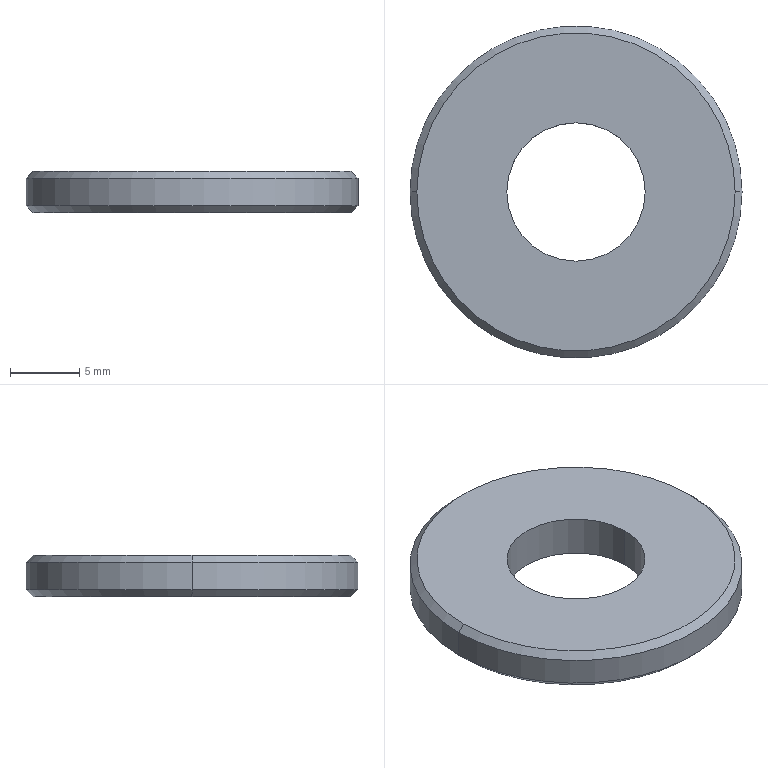Part | STEP file | VALVE_4PARTV11 | 1 solid | 10 faces | box 24 x 24 x 3 mm | volume 1103 mm3 | cone 4 | cylinder 4 | plane 2 | commonest cylinder face diameters 10 x2 24 x2
STEP:
#1=CARTESIAN_POINT('',(0.,0.,0.));
#2=DIRECTION('',(0.,0.,1.));
#3=DIRECTION('',(1.,0.,0.));
#4=AXIS2_PLACEMENT_3D('',#1,#2,#3);
#5=CARTESIAN_POINT('',(11.5,0.,3.));
#6=VERTEX_POINT('',#5);
#7=CARTESIAN_POINT('',(-11.5,0.,3.));
#8=VERTEX_POINT('',#7);
#9=CARTESIAN_POINT('',(0.,0.,3.));
#10=DIRECTION('',(0.,0.,1.));
#11=DIRECTION('',(1.,0.,0.));
#12=AXIS2_PLACEMENT_3D('',#9,#10,#11);
#13=CIRCLE('',#12,11.5);
#14=CARTESIAN_POINT('',(0.,0.,3.));
#15=DIRECTION('',(0.,0.,-1.));
#16=DIRECTION('',(-1.,0.,0.));
#17=AXIS2_PLACEMENT_3D('',#14,#15,#16);
#18=CONICAL_SURFACE('',#17,11.5,0.7854);
#19=CARTESIAN_POINT('',(3.142,0.));
#20=DIRECTION('',(-1.,0.));
#21=VECTOR('',#20,1.);
#22=LINE('',#19,#21);
#23=(GEOMETRIC_REPRESENTATION_CONTEXT(2)PARAMETRIC_REPRESENTATION_CONTEXT()REPRESENTATION_CONTEXT('',''));
#24=DEFINITIONAL_REPRESENTATION('',(#22),#23);
#25=PCURVE('',#18,#24);
#26=CARTESIAN_POINT('',(0.,0.,3.));
#27=DIRECTION('',(0.,0.,1.));
#28=DIRECTION('',(1.,0.,0.));
#29=AXIS2_PLACEMENT_3D('',#26,#27,#28);
#30=PLANE('',#29);
#31=CARTESIAN_POINT('',(0.,0.));
#32=DIRECTION('',(1.,0.));
#33=AXIS2_PLACEMENT_2D('',#31,#32);
#34=CIRCLE('',#33,11.5);
#35=(GEOMETRIC_REPRESENTATION_CONTEXT(2)PARAMETRIC_REPRESENTATION_CONTEXT()REPRESENTATION_CONTEXT('',''));
#36=DEFINITIONAL_REPRESENTATION('',(#34),#35);
#37=PCURVE('',#30,#36);
#38=SURFACE_CURVE('',#13,(#25,#37),.PCURVE_S1.);
#39=EDGE_CURVE('',#6,#8,#38,.T.);
#40=ORIENTED_EDGE('',*,*,#39,.F.);
#41=CARTESIAN_POINT('',(12.,0.,2.5));
#42=VERTEX_POINT('',#41);
#43=CARTESIAN_POINT('',(11.5,0.,3.));
#44=DIRECTION('',(0.7071,0.,-0.7071));
#45=VECTOR('',#44,1.);
#46=LINE('',#43,#45);
#47=CARTESIAN_POINT('',(3.142,0.));
#48=DIRECTION('',(0.,1.));
#49=VECTOR('',#48,1.);
#50=LINE('',#47,#49);
#51=(GEOMETRIC_REPRESENTATION_CONTEXT(2)PARAMETRIC_REPRESENTATION_CONTEXT()REPRESENTATION_CONTEXT('',''));
#52=DEFINITIONAL_REPRESENTATION('',(#50),#51);
#53=PCURVE('',#18,#52);
#54=CARTESIAN_POINT('',(0.,0.,3.));
#55=DIRECTION('',(0.,0.,-1.));
#56=DIRECTION('',(-1.,0.,0.));
#57=AXIS2_PLACEMENT_3D('',#54,#55,#56);
#58=CONICAL_SURFACE('',#57,11.5,0.7854);
#59=CARTESIAN_POINT('',(3.142,0.));
#60=DIRECTION('',(0.,1.));
#61=VECTOR('',#60,1.);
#62=LINE('',#59,#61);
#63=(GEOMETRIC_REPRESENTATION_CONTEXT(2)PARAMETRIC_REPRESENTATION_CONTEXT()REPRESENTATION_CONTEXT('',''));
#64=DEFINITIONAL_REPRESENTATION('',(#62),#63);
#65=PCURVE('',#58,#64);
#66=SURFACE_CURVE('',#46,(#53,#65),.PCURVE_S1.);
#67=EDGE_CURVE('',#6,#42,#66,.T.);
#68=ORIENTED_EDGE('',*,*,#67,.T.);
#69=CARTESIAN_POINT('',(-12.,0.,2.5));
#70=VERTEX_POINT('',#69);
#71=CARTESIAN_POINT('',(0.,0.,2.5));
#72=DIRECTION('',(0.,0.,-1.));
#73=DIRECTION('',(1.,0.,0.));
#74=AXIS2_PLACEMENT_3D('',#71,#72,#73);
#75=CIRCLE('',#74,12.);
#76=CARTESIAN_POINT('',(-3.142,0.5));
#77=DIRECTION('',(1.,0.));
#78=VECTOR('',#77,1.);
#79=LINE('',#76,#78);
#80=(GEOMETRIC_REPRESENTATION_CONTEXT(2)PARAMETRIC_REPRESENTATION_CONTEXT()REPRESENTATION_CONTEXT('',''));
#81=DEFINITIONAL_REPRESENTATION('',(#79),#80);
#82=PCURVE('',#18,#81);
#83=CARTESIAN_POINT('',(0.,0.,3.));
#84=DIRECTION('',(0.,0.,-1.));
#85=DIRECTION('',(-1.,0.,0.));
#86=AXIS2_PLACEMENT_3D('',#83,#84,#85);
#87=CYLINDRICAL_SURFACE('',#86,12.);
#88=CARTESIAN_POINT('',(-3.142,0.5));
#89=DIRECTION('',(1.,0.));
#90=VECTOR('',#89,1.);
#91=LINE('',#88,#90);
#92=(GEOMETRIC_REPRESENTATION_CONTEXT(2)PARAMETRIC_REPRESENTATION_CONTEXT()REPRESENTATION_CONTEXT('',''));
#93=DEFINITIONAL_REPRESENTATION('',(#91),#92);
#94=PCURVE('',#87,#93);
#95=SURFACE_CURVE('',#75,(#82,#94),.PCURVE_S1.);
#96=EDGE_CURVE('',#70,#42,#95,.T.);
#97=ORIENTED_EDGE('',*,*,#96,.F.);
#98=CARTESIAN_POINT('',(-11.5,0.,3.));
#99=DIRECTION('',(-0.7071,0.,-0.7071));
#100=VECTOR('',#99,1.);
#101=LINE('',#98,#100);
#102=CARTESIAN_POINT('',(0.,0.));
#103=DIRECTION('',(0.,1.));
#104=VECTOR('',#103,1.);
#105=LINE('',#102,#104);
#106=(GEOMETRIC_REPRESENTATION_CONTEXT(2)PARAMETRIC_REPRESENTATION_CONTEXT()REPRESENTATION_CONTEXT('',''));
#107=DEFINITIONAL_REPRESENTATION('',(#105),#106);
#108=PCURVE('',#18,#107);
#109=CARTESIAN_POINT('',(6.283,0.));
#110=DIRECTION('',(0.,1.));
#111=VECTOR('',#110,1.);
#112=LINE('',#109,#111);
#113=(GEOMETRIC_REPRESENTATION_CONTEXT(2)PARAMETRIC_REPRESENTATION_CONTEXT()REPRESENTATION_CONTEXT('',''));
#114=DEFINITIONAL_REPRESENTATION('',(#112),#113);
#115=PCURVE('',#58,#114);
#116=SURFACE_CURVE('',#101,(#108,#115),.PCURVE_S1.);
#117=EDGE_CURVE('',#8,#70,#116,.T.);
#118=ORIENTED_EDGE('',*,*,#117,.F.);
#119=EDGE_LOOP('',(#40,#68,#97,#118));
#120=FACE_BOUND('',#119,.T.);
#121=ADVANCED_FACE('',(#120),#18,.T.);
#122=CARTESIAN_POINT('',(-11.5,0.,0.));
#123=VERTEX_POINT('',#122);
#124=CARTESIAN_POINT('',(11.5,0.,0.));
#125=VERTEX_POINT('',#124);
#126=CARTESIAN_POINT('',(0.,0.,0.));
#127=DIRECTION('',(0.,0.,-1.));
#128=DIRECTION('',(1.,0.,0.));
#129=AXIS2_PLACEMENT_3D('',#126,#127,#128);
#130=CIRCLE('',#129,11.5);
#131=CARTESIAN_POINT('',(0.,0.,0.5));
#132=DIRECTION('',(0.,0.,1.));
#133=DIRECTION('',(1.,0.,0.));
#134=AXIS2_PLACEMENT_3D('',#131,#132,#133);
#135=CONICAL_SURFACE('',#134,12.,0.7854);
#136=CARTESIAN_POINT('',(6.283,-0.5));
#137=DIRECTION('',(-1.,0.));
#138=VECTOR('',#137,1.);
#139=LINE('',#136,#138);
#140=(GEOMETRIC_REPRESENTATION_CONTEXT(2)PARAMETRIC_REPRESENTATION_CONTEXT()REPRESENTATION_CONTEXT('',''));
#141=DEFINITIONAL_REPRESENTATION('',(#139),#140);
#142=PCURVE('',#135,#141);
#143=CARTESIAN_POINT('',(0.,0.,0.));
#144=DIRECTION('',(0.,0.,1.));
#145=DIRECTION('',(1.,0.,0.));
#146=AXIS2_PLACEMENT_3D('',#143,#144,#145);
#147=PLANE('',#146);
#148=CARTESIAN_POINT('',(11.5,0.));
#149=CARTESIAN_POINT('',(11.5,-19.919));
#150=CARTESIAN_POINT('',(-5.75,-9.959));
#151=CARTESIAN_POINT('',(-23.,0.));
#152=CARTESIAN_POINT('',(-5.75,9.959));
#153=CARTESIAN_POINT('',(11.5,19.919));
#154=CARTESIAN_POINT('',(11.5,0.));
#155=(BOUNDED_CURVE()B_SPLINE_CURVE(2,(#148,#149,#150,#151,#152,#153,#154),.UNSPECIFIED.,.T.,.F.)B_SPLINE_CURVE_WITH_KNOTS((1,2,2,2,2,1),(-2.094,0.,2.094,4.189,6.283,8.378),.UNSPECIFIED.)CURVE()GEOMETRIC_REPRESENTATION_ITEM()RATIONAL_B_SPLINE_CURVE((1.,0.5,1.,0.5,1.,0.5,1.))REPRESENTATION_ITEM(''));
#156=(GEOMETRIC_REPRESENTATION_CONTEXT(2)PARAMETRIC_REPRESENTATION_CONTEXT()REPRESENTATION_CONTEXT('',''));
#157=DEFINITIONAL_REPRESENTATION('',(#155),#156);
#158=PCURVE('',#147,#157);
#159=SURFACE_CURVE('',#130,(#142,#158),.PCURVE_S1.);
#160=EDGE_CURVE('',#123,#125,#159,.T.);
#161=ORIENTED_EDGE('',*,*,#160,.F.);
#162=CARTESIAN_POINT('',(-12.,0.,0.5));
#163=VERTEX_POINT('',#162);
#164=CARTESIAN_POINT('',(-12.,0.,0.5));
#165=DIRECTION('',(-0.7071,0.,0.7071));
#166=VECTOR('',#165,1.);
#167=LINE('',#164,#166);
#168=CARTESIAN_POINT('',(3.142,0.));
#169=DIRECTION('',(0.,1.));
#170=VECTOR('',#169,1.);
#171=LINE('',#168,#170);
#172=(GEOMETRIC_REPRESENTATION_CONTEXT(2)PARAMETRIC_REPRESENTATION_CONTEXT()REPRESENTATION_CONTEXT('',''));
#173=DEFINITIONAL_REPRESENTATION('',(#171),#172);
#174=PCURVE('',#135,#173);
#175=CARTESIAN_POINT('',(0.,0.,0.5));
#176=DIRECTION('',(0.,0.,1.));
#177=DIRECTION('',(1.,0.,0.));
#178=AXIS2_PLACEMENT_3D('',#175,#176,#177);
#179=CONICAL_SURFACE('',#178,12.,0.7854);
#180=CARTESIAN_POINT('',(3.142,0.));
#181=DIRECTION('',(0.,1.));
#182=VECTOR('',#181,1.);
#183=LINE('',#180,#182);
#184=(GEOMETRIC_REPRESENTATION_CONTEXT(2)PARAMETRIC_REPRESENTATION_CONTEXT()REPRESENTATION_CONTEXT('',''));
#185=DEFINITIONAL_REPRESENTATION('',(#183),#184);
#186=PCURVE('',#179,#185);
#187=SURFACE_CURVE('',#167,(#174,#186),.PCURVE_S1.);
#188=EDGE_CURVE('',#123,#163,#187,.T.);
#189=ORIENTED_EDGE('',*,*,#188,.T.);
#190=CARTESIAN_POINT('',(12.,0.,0.5));
#191=VERTEX_POINT('',#190);
#192=CARTESIAN_POINT('',(0.,0.,0.5));
#193=DIRECTION('',(0.,0.,1.));
#194=DIRECTION('',(1.,0.,0.));
#195=AXIS2_PLACEMENT_3D('',#192,#193,#194);
#196=CIRCLE('',#195,12.);
#197=CARTESIAN_POINT('',(0.,0.));
#198=DIRECTION('',(1.,0.));
#199=VECTOR('',#198,1.);
#200=LINE('',#197,#199);
#201=(GEOMETRIC_REPRESENTATION_CONTEXT(2)PARAMETRIC_REPRESENTATION_CONTEXT()REPRESENTATION_CONTEXT('',''));
#202=DEFINITIONAL_REPRESENTATION('',(#200),#201);
#203=PCURVE('',#135,#202);
#204=CARTESIAN_POINT('',(3.142,2.5));
#205=DIRECTION('',(-1.,0.));
#206=VECTOR('',#205,1.);
#207=LINE('',#204,#206);
#208=(GEOMETRIC_REPRESENTATION_CONTEXT(2)PARAMETRIC_REPRESENTATION_CONTEXT()REPRESENTATION_CONTEXT('',''));
#209=DEFINITIONAL_REPRESENTATION('',(#207),#208);
#210=PCURVE('',#87,#209);
#211=SURFACE_CURVE('',#196,(#203,#210),.PCURVE_S1.);
#212=EDGE_CURVE('',#191,#163,#211,.T.);
#213=ORIENTED_EDGE('',*,*,#212,.F.);
#214=CARTESIAN_POINT('',(12.,0.,0.5));
#215=DIRECTION('',(0.7071,0.,0.7071));
#216=VECTOR('',#215,1.);
#217=LINE('',#214,#216);
#218=CARTESIAN_POINT('',(0.,0.));
#219=DIRECTION('',(0.,1.));
#220=VECTOR('',#219,1.);
#221=LINE('',#218,#220);
#222=(GEOMETRIC_REPRESENTATION_CONTEXT(2)PARAMETRIC_REPRESENTATION_CONTEXT()REPRESENTATION_CONTEXT('',''));
#223=DEFINITIONAL_REPRESENTATION('',(#221),#222);
#224=PCURVE('',#135,#223);
#225=CARTESIAN_POINT('',(6.283,0.));
#226=DIRECTION('',(0.,1.));
#227=VECTOR('',#226,1.);
#228=LINE('',#225,#227);
#229=(GEOMETRIC_REPRESENTATION_CONTEXT(2)PARAMETRIC_REPRESENTATION_CONTEXT()REPRESENTATION_CONTEXT('',''));
#230=DEFINITIONAL_REPRESENTATION('',(#228),#229);
#231=PCURVE('',#179,#230);
#232=SURFACE_CURVE('',#217,(#224,#231),.PCURVE_S1.);
#233=EDGE_CURVE('',#125,#191,#232,.T.);
#234=ORIENTED_EDGE('',*,*,#233,.F.);
#235=EDGE_LOOP('',(#161,#189,#213,#234));
#236=FACE_BOUND('',#235,.T.);
#237=ADVANCED_FACE('',(#236),#135,.T.);
#238=CARTESIAN_POINT('',(-5.,0.,3.));
#239=VERTEX_POINT('',#238);
#240=CARTESIAN_POINT('',(-5.,0.,0.));
#241=VERTEX_POINT('',#240);
#242=CARTESIAN_POINT('',(-5.,0.,3.));
#243=DIRECTION('',(0.,0.,-1.));
#244=VECTOR('',#243,1.);
#245=LINE('',#242,#244);
#246=CARTESIAN_POINT('',(0.,0.,3.));
#247=DIRECTION('',(0.,0.,-1.));
#248=DIRECTION('',(-1.,0.,0.));
#249=AXIS2_PLACEMENT_3D('',#246,#247,#248);
#250=CYLINDRICAL_SURFACE('',#249,5.);
#251=CARTESIAN_POINT('',(6.283,0.));
#252=DIRECTION('',(0.,1.));
#253=VECTOR('',#252,1.);
#254=LINE('',#251,#253);
#255=(GEOMETRIC_REPRESENTATION_CONTEXT(2)PARAMETRIC_REPRESENTATION_CONTEXT()REPRESENTATION_CONTEXT('',''));
#256=DEFINITIONAL_REPRESENTATION('',(#254),#255);
#257=PCURVE('',#250,#256);
#258=CARTESIAN_POINT('',(0.,0.,3.));
#259=DIRECTION('',(0.,0.,-1.));
#260=DIRECTION('',(-1.,0.,0.));
#261=AXIS2_PLACEMENT_3D('',#258,#259,#260);
#262=CYLINDRICAL_SURFACE('',#261,5.);
#263=CARTESIAN_POINT('',(0.,0.));
#264=DIRECTION('',(0.,1.));
#265=VECTOR('',#264,1.);
#266=LINE('',#263,#265);
#267=(GEOMETRIC_REPRESENTATION_CONTEXT(2)PARAMETRIC_REPRESENTATION_CONTEXT()REPRESENTATION_CONTEXT('',''));
#268=DEFINITIONAL_REPRESENTATION('',(#266),#267);
#269=PCURVE('',#262,#268);
#270=SURFACE_CURVE('',#245,(#257,#269),.PCURVE_S1.);
#271=EDGE_CURVE('',#239,#241,#270,.T.);
#272=ORIENTED_EDGE('',*,*,#271,.T.);
#273=CARTESIAN_POINT('',(5.,0.,0.));
#274=VERTEX_POINT('',#273);
#275=CARTESIAN_POINT('',(0.,0.,0.));
#276=DIRECTION('',(0.,0.,1.));
#277=DIRECTION('',(1.,0.,0.));
#278=AXIS2_PLACEMENT_3D('',#275,#276,#277);
#279=CIRCLE('',#278,5.);
#280=CARTESIAN_POINT('',(9.425,3.));
#281=DIRECTION('',(-1.,0.));
#282=VECTOR('',#281,1.);
#283=LINE('',#280,#282);
#284=(GEOMETRIC_REPRESENTATION_CONTEXT(2)PARAMETRIC_REPRESENTATION_CONTEXT()REPRESENTATION_CONTEXT('',''));
#285=DEFINITIONAL_REPRESENTATION('',(#283),#284);
#286=PCURVE('',#250,#285);
#287=CARTESIAN_POINT('',(0.,0.));
#288=DIRECTION('',(1.,0.));
#289=AXIS2_PLACEMENT_2D('',#287,#288);
#290=CIRCLE('',#289,5.);
#291=(GEOMETRIC_REPRESENTATION_CONTEXT(2)PARAMETRIC_REPRESENTATION_CONTEXT()REPRESENTATION_CONTEXT('',''));
#292=DEFINITIONAL_REPRESENTATION('',(#290),#291);
#293=PCURVE('',#147,#292);
#294=SURFACE_CURVE('',#279,(#286,#293),.PCURVE_S1.);
#295=EDGE_CURVE('',#241,#274,#294,.T.);
#296=ORIENTED_EDGE('',*,*,#295,.T.);
#297=CARTESIAN_POINT('',(5.,0.,3.));
#298=VERTEX_POINT('',#297);
#299=CARTESIAN_POINT('',(5.,0.,3.));
#300=DIRECTION('',(0.,0.,-1.));
#301=VECTOR('',#300,1.);
#302=LINE('',#299,#301);
#303=CARTESIAN_POINT('',(3.142,0.));
#304=DIRECTION('',(0.,1.));
#305=VECTOR('',#304,1.);
#306=LINE('',#303,#305);
#307=(GEOMETRIC_REPRESENTATION_CONTEXT(2)PARAMETRIC_REPRESENTATION_CONTEXT()REPRESENTATION_CONTEXT('',''));
#308=DEFINITIONAL_REPRESENTATION('',(#306),#307);
#309=PCURVE('',#250,#308);
#310=CARTESIAN_POINT('',(3.142,0.));
#311=DIRECTION('',(0.,1.));
#312=VECTOR('',#311,1.);
#313=LINE('',#310,#312);
#314=(GEOMETRIC_REPRESENTATION_CONTEXT(2)PARAMETRIC_REPRESENTATION_CONTEXT()REPRESENTATION_CONTEXT('',''));
#315=DEFINITIONAL_REPRESENTATION('',(#313),#314);
#316=PCURVE('',#262,#315);
#317=SURFACE_CURVE('',#302,(#309,#316),.PCURVE_S1.);
#318=EDGE_CURVE('',#298,#274,#317,.T.);
#319=ORIENTED_EDGE('',*,*,#318,.F.);
#320=CARTESIAN_POINT('',(0.,0.,3.));
#321=DIRECTION('',(0.,0.,1.));
#322=DIRECTION('',(1.,0.,0.));
#323=AXIS2_PLACEMENT_3D('',#320,#321,#322);
#324=CIRCLE('',#323,5.);
#325=CARTESIAN_POINT('',(9.425,0.));
#326=DIRECTION('',(-1.,0.));
#327=VECTOR('',#326,1.);
#328=LINE('',#325,#327);
#329=(GEOMETRIC_REPRESENTATION_CONTEXT(2)PARAMETRIC_REPRESENTATION_CONTEXT()REPRESENTATION_CONTEXT('',''));
#330=DEFINITIONAL_REPRESENTATION('',(#328),#329);
#331=PCURVE('',#250,#330);
#332=CARTESIAN_POINT('',(0.,0.));
#333=DIRECTION('',(1.,0.));
#334=AXIS2_PLACEMENT_2D('',#332,#333);
#335=CIRCLE('',#334,5.);
#336=(GEOMETRIC_REPRESENTATION_CONTEXT(2)PARAMETRIC_REPRESENTATION_CONTEXT()REPRESENTATION_CONTEXT('',''));
#337=DEFINITIONAL_REPRESENTATION('',(#335),#336);
#338=PCURVE('',#30,#337);
#339=SURFACE_CURVE('',#324,(#331,#338),.PCURVE_S1.);
#340=EDGE_CURVE('',#239,#298,#339,.T.);
#341=ORIENTED_EDGE('',*,*,#340,.F.);
#342=EDGE_LOOP('',(#272,#296,#319,#341));
#343=FACE_BOUND('',#342,.F.);
#344=ADVANCED_FACE('',(#343),#250,.F.);
#345=ORIENTED_EDGE('',*,*,#96,.T.);
#346=CARTESIAN_POINT('',(12.,0.,3.));
#347=DIRECTION('',(0.,0.,-1.));
#348=VECTOR('',#347,1.);
#349=LINE('',#346,#348);
#350=CARTESIAN_POINT('',(3.142,0.));
#351=DIRECTION('',(0.,1.));
#352=VECTOR('',#351,1.);
#353=LINE('',#350,#352);
#354=(GEOMETRIC_REPRESENTATION_CONTEXT(2)PARAMETRIC_REPRESENTATION_CONTEXT()REPRESENTATION_CONTEXT('',''));
#355=DEFINITIONAL_REPRESENTATION('',(#353),#354);
#356=PCURVE('',#87,#355);
#357=CARTESIAN_POINT('',(0.,0.,3.));
#358=DIRECTION('',(0.,0.,-1.));
#359=DIRECTION('',(-1.,0.,0.));
#360=AXIS2_PLACEMENT_3D('',#357,#358,#359);
#361=CYLINDRICAL_SURFACE('',#360,12.);
#362=CARTESIAN_POINT('',(3.142,0.));
#363=DIRECTION('',(0.,1.));
#364=VECTOR('',#363,1.);
#365=LINE('',#362,#364);
#366=(GEOMETRIC_REPRESENTATION_CONTEXT(2)PARAMETRIC_REPRESENTATION_CONTEXT()REPRESENTATION_CONTEXT('',''));
#367=DEFINITIONAL_REPRESENTATION('',(#365),#366);
#368=PCURVE('',#361,#367);
#369=SURFACE_CURVE('',#349,(#356,#368),.PCURVE_S1.);
#370=EDGE_CURVE('',#42,#191,#369,.T.);
#371=ORIENTED_EDGE('',*,*,#370,.T.);
#372=ORIENTED_EDGE('',*,*,#212,.T.);
#373=CARTESIAN_POINT('',(-12.,0.,3.));
#374=DIRECTION('',(0.,0.,-1.));
#375=VECTOR('',#374,1.);
#376=LINE('',#373,#375);
#377=CARTESIAN_POINT('',(0.,0.));
#378=DIRECTION('',(0.,1.));
#379=VECTOR('',#378,1.);
#380=LINE('',#377,#379);
#381=(GEOMETRIC_REPRESENTATION_CONTEXT(2)PARAMETRIC_REPRESENTATION_CONTEXT()REPRESENTATION_CONTEXT('',''));
#382=DEFINITIONAL_REPRESENTATION('',(#380),#381);
#383=PCURVE('',#87,#382);
#384=CARTESIAN_POINT('',(6.283,0.));
#385=DIRECTION('',(0.,1.));
#386=VECTOR('',#385,1.);
#387=LINE('',#384,#386);
#388=(GEOMETRIC_REPRESENTATION_CONTEXT(2)PARAMETRIC_REPRESENTATION_CONTEXT()REPRESENTATION_CONTEXT('',''));
#389=DEFINITIONAL_REPRESENTATION('',(#387),#388);
#390=PCURVE('',#361,#389);
#391=SURFACE_CURVE('',#376,(#383,#390),.PCURVE_S1.);
#392=EDGE_CURVE('',#70,#163,#391,.T.);
#393=ORIENTED_EDGE('',*,*,#392,.F.);
#394=EDGE_LOOP('',(#345,#371,#372,#393));
#395=FACE_BOUND('',#394,.T.);
#396=ADVANCED_FACE('',(#395),#87,.T.);
#397=CARTESIAN_POINT('',(0.,0.,3.));
#398=DIRECTION('',(0.,0.,1.));
#399=DIRECTION('',(1.,0.,0.));
#400=AXIS2_PLACEMENT_3D('',#397,#398,#399);
#401=CIRCLE('',#400,11.5);
#402=CARTESIAN_POINT('',(0.,0.));
#403=DIRECTION('',(1.,0.));
#404=AXIS2_PLACEMENT_2D('',#402,#403);
#405=CIRCLE('',#404,11.5);
#406=(GEOMETRIC_REPRESENTATION_CONTEXT(2)PARAMETRIC_REPRESENTATION_CONTEXT()REPRESENTATION_CONTEXT('',''));
#407=DEFINITIONAL_REPRESENTATION('',(#405),#406);
#408=PCURVE('',#30,#407);
#409=CARTESIAN_POINT('',(9.425,0.));
#410=DIRECTION('',(-1.,0.));
#411=VECTOR('',#410,1.);
#412=LINE('',#409,#411);
#413=(GEOMETRIC_REPRESENTATION_CONTEXT(2)PARAMETRIC_REPRESENTATION_CONTEXT()REPRESENTATION_CONTEXT('',''));
#414=DEFINITIONAL_REPRESENTATION('',(#412),#413);
#415=PCURVE('',#58,#414);
#416=SURFACE_CURVE('',#401,(#408,#415),.PCURVE_S1.);
#417=EDGE_CURVE('',#8,#6,#416,.T.);
#418=ORIENTED_EDGE('',*,*,#417,.T.);
#419=ORIENTED_EDGE('',*,*,#39,.T.);
#420=EDGE_LOOP('',(#418,#419));
#421=FACE_BOUND('',#420,.T.);
#422=ORIENTED_EDGE('',*,*,#340,.F.);
#423=CARTESIAN_POINT('',(0.,0.,3.));
#424=DIRECTION('',(0.,0.,1.));
#425=DIRECTION('',(1.,0.,0.));
#426=AXIS2_PLACEMENT_3D('',#423,#424,#425);
#427=CIRCLE('',#426,5.);
#428=CARTESIAN_POINT('',(0.,0.));
#429=DIRECTION('',(1.,0.));
#430=AXIS2_PLACEMENT_2D('',#428,#429);
#431=CIRCLE('',#430,5.);
#432=(GEOMETRIC_REPRESENTATION_CONTEXT(2)PARAMETRIC_REPRESENTATION_CONTEXT()REPRESENTATION_CONTEXT('',''));
#433=DEFINITIONAL_REPRESENTATION('',(#431),#432);
#434=PCURVE('',#30,#433);
#435=CARTESIAN_POINT('',(3.142,0.));
#436=DIRECTION('',(-1.,0.));
#437=VECTOR('',#436,1.);
#438=LINE('',#435,#437);
#439=(GEOMETRIC_REPRESENTATION_CONTEXT(2)PARAMETRIC_REPRESENTATION_CONTEXT()REPRESENTATION_CONTEXT('',''));
#440=DEFINITIONAL_REPRESENTATION('',(#438),#439);
#441=PCURVE('',#262,#440);
#442=SURFACE_CURVE('',#427,(#434,#441),.PCURVE_S1.);
#443=EDGE_CURVE('',#298,#239,#442,.T.);
#444=ORIENTED_EDGE('',*,*,#443,.F.);
#445=EDGE_LOOP('',(#422,#444));
#446=FACE_BOUND('',#445,.T.);
#447=ADVANCED_FACE('',(#421,#446),#30,.T.);
#448=CARTESIAN_POINT('',(0.,0.,0.));
#449=DIRECTION('',(0.,0.,-1.));
#450=DIRECTION('',(1.,0.,0.));
#451=AXIS2_PLACEMENT_3D('',#448,#449,#450);
#452=CIRCLE('',#451,11.5);
#453=CARTESIAN_POINT('',(11.5,0.));
#454=CARTESIAN_POINT('',(11.5,-19.919));
#455=CARTESIAN_POINT('',(-5.75,-9.959));
#456=CARTESIAN_POINT('',(-23.,0.));
#457=CARTESIAN_POINT('',(-5.75,9.959));
#458=CARTESIAN_POINT('',(11.5,19.919));
#459=CARTESIAN_POINT('',(11.5,0.));
#460=(BOUNDED_CURVE()B_SPLINE_CURVE(2,(#453,#454,#455,#456,#457,#458,#459),.UNSPECIFIED.,.T.,.F.)B_SPLINE_CURVE_WITH_KNOTS((1,2,2,2,2,1),(-2.094,0.,2.094,4.189,6.283,8.378),.UNSPECIFIED.)CURVE()GEOMETRIC_REPRESENTATION_ITEM()RATIONAL_B_SPLINE_CURVE((1.,0.5,1.,0.5,1.,0.5,1.))REPRESENTATION_ITEM(''));
#461=(GEOMETRIC_REPRESENTATION_CONTEXT(2)PARAMETRIC_REPRESENTATION_CONTEXT()REPRESENTATION_CONTEXT('',''));
#462=DEFINITIONAL_REPRESENTATION('',(#460),#461);
#463=PCURVE('',#147,#462);
#464=CARTESIAN_POINT('',(6.283,-0.5));
#465=DIRECTION('',(-1.,0.));
#466=VECTOR('',#465,1.);
#467=LINE('',#464,#466);
#468=(GEOMETRIC_REPRESENTATION_CONTEXT(2)PARAMETRIC_REPRESENTATION_CONTEXT()REPRESENTATION_CONTEXT('',''));
#469=DEFINITIONAL_REPRESENTATION('',(#467),#468);
#470=PCURVE('',#179,#469);
#471=SURFACE_CURVE('',#452,(#463,#470),.PCURVE_S1.);
#472=EDGE_CURVE('',#125,#123,#471,.T.);
#473=ORIENTED_EDGE('',*,*,#472,.T.);
#474=ORIENTED_EDGE('',*,*,#160,.T.);
#475=EDGE_LOOP('',(#473,#474));
#476=FACE_BOUND('',#475,.T.);
#477=ORIENTED_EDGE('',*,*,#295,.T.);
#478=CARTESIAN_POINT('',(0.,0.,0.));
#479=DIRECTION('',(0.,0.,1.));
#480=DIRECTION('',(1.,0.,0.));
#481=AXIS2_PLACEMENT_3D('',#478,#479,#480);
#482=CIRCLE('',#481,5.);
#483=CARTESIAN_POINT('',(0.,0.));
#484=DIRECTION('',(1.,0.));
#485=AXIS2_PLACEMENT_2D('',#483,#484);
#486=CIRCLE('',#485,5.);
#487=(GEOMETRIC_REPRESENTATION_CONTEXT(2)PARAMETRIC_REPRESENTATION_CONTEXT()REPRESENTATION_CONTEXT('',''));
#488=DEFINITIONAL_REPRESENTATION('',(#486),#487);
#489=PCURVE('',#147,#488);
#490=CARTESIAN_POINT('',(3.142,3.));
#491=DIRECTION('',(-1.,0.));
#492=VECTOR('',#491,1.);
#493=LINE('',#490,#492);
#494=(GEOMETRIC_REPRESENTATION_CONTEXT(2)PARAMETRIC_REPRESENTATION_CONTEXT()REPRESENTATION_CONTEXT('',''));
#495=DEFINITIONAL_REPRESENTATION('',(#493),#494);
#496=PCURVE('',#262,#495);
#497=SURFACE_CURVE('',#482,(#489,#496),.PCURVE_S1.);
#498=EDGE_CURVE('',#274,#241,#497,.T.);
#499=ORIENTED_EDGE('',*,*,#498,.T.);
#500=EDGE_LOOP('',(#477,#499));
#501=FACE_BOUND('',#500,.T.);
#502=ADVANCED_FACE('',(#476,#501),#147,.F.);
#503=ORIENTED_EDGE('',*,*,#370,.F.);
#504=CARTESIAN_POINT('',(0.,0.,2.5));
#505=DIRECTION('',(0.,0.,-1.));
#506=DIRECTION('',(1.,0.,0.));
#507=AXIS2_PLACEMENT_3D('',#504,#505,#506);
#508=CIRCLE('',#507,12.);
#509=CARTESIAN_POINT('',(3.142,0.5));
#510=DIRECTION('',(1.,0.));
#511=VECTOR('',#510,1.);
#512=LINE('',#509,#511);
#513=(GEOMETRIC_REPRESENTATION_CONTEXT(2)PARAMETRIC_REPRESENTATION_CONTEXT()REPRESENTATION_CONTEXT('',''));
#514=DEFINITIONAL_REPRESENTATION('',(#512),#513);
#515=PCURVE('',#361,#514);
#516=CARTESIAN_POINT('',(3.142,0.5));
#517=DIRECTION('',(1.,0.));
#518=VECTOR('',#517,1.);
#519=LINE('',#516,#518);
#520=(GEOMETRIC_REPRESENTATION_CONTEXT(2)PARAMETRIC_REPRESENTATION_CONTEXT()REPRESENTATION_CONTEXT('',''));
#521=DEFINITIONAL_REPRESENTATION('',(#519),#520);
#522=PCURVE('',#58,#521);
#523=SURFACE_CURVE('',#508,(#515,#522),.PCURVE_S1.);
#524=EDGE_CURVE('',#42,#70,#523,.T.);
#525=ORIENTED_EDGE('',*,*,#524,.T.);
#526=ORIENTED_EDGE('',*,*,#392,.T.);
#527=CARTESIAN_POINT('',(0.,0.,0.5));
#528=DIRECTION('',(0.,0.,1.));
#529=DIRECTION('',(1.,0.,0.));
#530=AXIS2_PLACEMENT_3D('',#527,#528,#529);
#531=CIRCLE('',#530,12.);
#532=CARTESIAN_POINT('',(9.425,2.5));
#533=DIRECTION('',(-1.,0.));
#534=VECTOR('',#533,1.);
#535=LINE('',#532,#534);
#536=(GEOMETRIC_REPRESENTATION_CONTEXT(2)PARAMETRIC_REPRESENTATION_CONTEXT()REPRESENTATION_CONTEXT('',''));
#537=DEFINITIONAL_REPRESENTATION('',(#535),#536);
#538=PCURVE('',#361,#537);
#539=CARTESIAN_POINT('',(0.,0.));
#540=DIRECTION('',(1.,0.));
#541=VECTOR('',#540,1.);
#542=LINE('',#539,#541);
#543=(GEOMETRIC_REPRESENTATION_CONTEXT(2)PARAMETRIC_REPRESENTATION_CONTEXT()REPRESENTATION_CONTEXT('',''));
#544=DEFINITIONAL_REPRESENTATION('',(#542),#543);
#545=PCURVE('',#179,#544);
#546=SURFACE_CURVE('',#531,(#538,#545),.PCURVE_S1.);
#547=EDGE_CURVE('',#163,#191,#546,.T.);
#548=ORIENTED_EDGE('',*,*,#547,.T.);
#549=EDGE_LOOP('',(#503,#525,#526,#548));
#550=FACE_BOUND('',#549,.T.);
#551=ADVANCED_FACE('',(#550),#361,.T.);
#552=ORIENTED_EDGE('',*,*,#498,.T.);
#553=ORIENTED_EDGE('',*,*,#271,.F.);
#554=ORIENTED_EDGE('',*,*,#443,.F.);
#555=ORIENTED_EDGE('',*,*,#318,.T.);
#556=EDGE_LOOP('',(#552,#553,#554,#555));
#557=FACE_BOUND('',#556,.F.);
#558=ADVANCED_FACE('',(#557),#262,.F.);
#559=ORIENTED_EDGE('',*,*,#188,.F.);
#560=ORIENTED_EDGE('',*,*,#472,.F.);
#561=ORIENTED_EDGE('',*,*,#233,.T.);
#562=ORIENTED_EDGE('',*,*,#547,.F.);
#563=EDGE_LOOP('',(#559,#560,#561,#562));
#564=FACE_BOUND('',#563,.T.);
#565=ADVANCED_FACE('',(#564),#179,.T.);
#566=ORIENTED_EDGE('',*,*,#67,.F.);
#567=ORIENTED_EDGE('',*,*,#417,.F.);
#568=ORIENTED_EDGE('',*,*,#117,.T.);
#569=ORIENTED_EDGE('',*,*,#524,.F.);
#570=EDGE_LOOP('',(#566,#567,#568,#569));
#571=FACE_BOUND('',#570,.T.);
#572=ADVANCED_FACE('',(#571),#58,.T.);
#573=CLOSED_SHELL('',(#121,#237,#344,#396,#447,#502,#551,#558,#565,#572));
#574=MANIFOLD_SOLID_BREP('',#573);
#575=(LENGTH_UNIT()NAMED_UNIT(*)SI_UNIT(.MILLI.,.METRE.));
#576=UNCERTAINTY_MEASURE_WITH_UNIT(LENGTH_MEASURE(0.0000001),#575,'','');
#577=(NAMED_UNIT(*)PLANE_ANGLE_UNIT()SI_UNIT($,.RADIAN.));
#578=(NAMED_UNIT(*)SI_UNIT($,.STERADIAN.)SOLID_ANGLE_UNIT());
#579=(GEOMETRIC_REPRESENTATION_CONTEXT(3)GLOBAL_UNCERTAINTY_ASSIGNED_CONTEXT((#576))GLOBAL_UNIT_ASSIGNED_CONTEXT((#575,#577,#578))REPRESENTATION_CONTEXT('',''));
#580=ADVANCED_BREP_SHAPE_REPRESENTATION('',(#4,#574),#579);